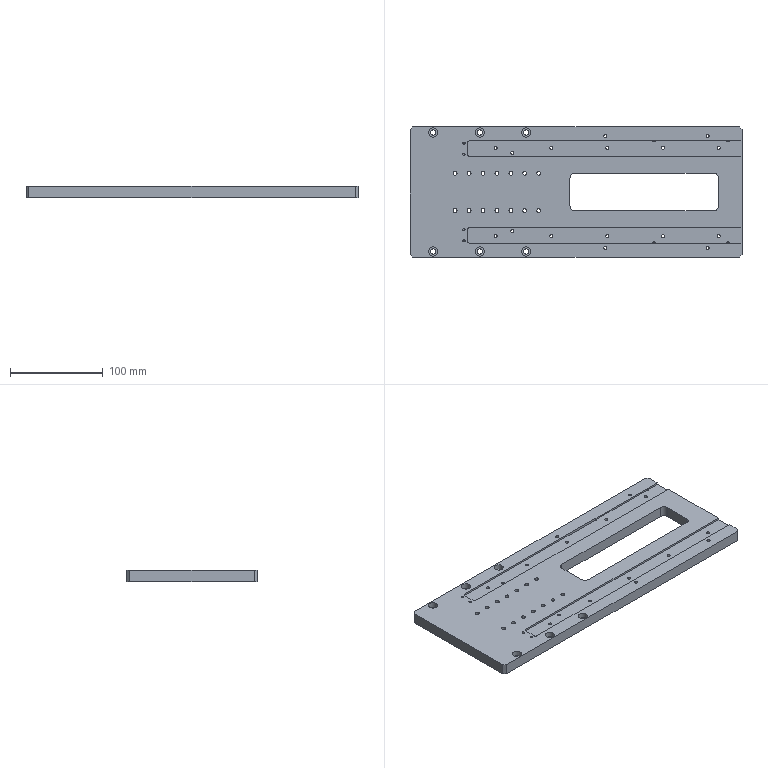NC program | NX | posted with a generic post | part box 357 x 140 x 12 mm
Lines 5825 to 6551 of 6551:
(PLANAR_MILL_COPY_COPY_COPY , TOOL : D6A45)
N11630 T01 M6
N11632 G54
N11634 G17 G0 G90 X-60.247 Y-0.314 B0. C0. S8500 M3
N11636 G43 Z30. H1
N11638 Z0.5
N11640 G94 G1 Z-1. F1250.
N11642 X-60.866 Y-1.1
N11644 G3 X-60. Y-1.6 R1.
N11646 X-58.4 Y0. R1.6
N11648 X-60. Y-1.6 R-1.6
N11650 X-59.134 Y-1.1 R1.
N11652 G1 X-59.753 Y-0.314
N11654 Z0.5
N11656 G0 Z30.
N11658 X-23.688 Y-0.13
N11660 Z0.5
N11662 G1 X-23.692 Y-0.302 Z0.454
N11664 X-23.358 Y-0.881 Z0.275
N11666 X-22.77 Y-1.2 Z0.095
N11668 X-22.23 Z-0.049
N11670 X-21.642 Y-0.881 Z-0.228
N11672 X-21.308 Y-0.302 Z-0.408
N11674 X-21.326 Y0.366 Z-0.587
N11676 X-21.596 Y0.834 Z-0.731
N11678 X-22.23 Y1.2 Z-0.928
N11680 X-22.5 Z-1.
N11682 G3 X-23.7 Y0. R1.2
N11684 X-22.5 Y1.2 R-1.2
N11686 X-23.366 Y0.7 R1.
N11688 G1 Z0.5
N11690 G0 Z30.
N11692 X23.688 Y0.13
N11694 Z0.5
N11696 G1 X23.692 Y0.302 Z0.454
N11698 X23.358 Y0.881 Z0.275
N11700 X22.77 Y1.2 Z0.095
N11702 X22.23 Z-0.049
N11704 X21.642 Y0.881 Z-0.228
N11706 X21.308 Y0.302 Z-0.408
N11708 X21.326 Y-0.366 Z-0.587
N11710 X21.596 Y-0.834 Z-0.731
N11712 X22.23 Y-1.2 Z-0.928
N11714 X22.5 Z-1.
N11716 G3 X23.7 Y0. R1.2
N11718 X22.5 Y-1.2 R-1.2
N11720 X23.366 Y-0.7 R1.
N11722 G1 Z0.5
N11724 G0 Z30.
N11726 X60.626 Y0.38
N11728 Z0.5
N11730 G1 Z-1.
N11732 X60.866 Y1.1
N11734 G3 X60. Y1.6 R1.
N11736 G1 X59.5
N11738 G3 X57.9 Y0. R1.6
N11740 X59.5 Y-1.6 R1.6
N11742 G1 X60.5
N11744 G3 X62.1 Y0. R1.6
N11746 X60.5 Y1.6 R1.6
N11748 G1 X60.
N11750 G3 X59.134 Y1.1 R1.
N11752 G1 X59.374 Y0.38
N11754 Z0.5
N11756 G0 Z30.
N11758 M5
(刀补 , TOOL : D3)
N11760 T16 M6
N11762 G54
N11764 G17 G0 G90 X-60.108 Y-0.333 B0. C0. S9500 M3
N11766 G43 Z30. H16
N11768 Z-1.
N11770 G94 G1 Z-2. F1000.
N11772 G41 X-60.26 Y-0.8 D16
N11774 G3 X-60. Y-0.95 R0.3
N11776 X-59.05 Y0. R0.95 F1200.
N11778 X-60. Y-0.95 R-0.95
N11780 G1 X-59.853 Y-0.932 Z-2.05
N11782 X-59.79 Y-0.917 Z-2.072
N11784 X-59.7 Y-0.894 Z-2.103
N11786 X-59.657 Y-0.878 Z-2.119
N11788 X-59.59 Y-0.847 Z-2.143
N11790 X-59.506 Y-0.803 Z-2.176
N11792 X-59.448 Y-0.762 Z-2.2
N11794 X-59.411 Y-0.736 Z-2.215
N11796 X-59.353 Y-0.683 Z-2.241
N11798 X-59.303 Y-0.633 Z-2.265
N11800 X-59.262 Y-0.585 Z-2.287
N11802 X-59.212 Y-0.515 Z-2.316
N11804 X-59.187 Y-0.479 Z-2.331
N11806 X-59.173 Y-0.453 Z-2.341
N11808 X-59.147 Y-0.398 Z-2.361
N11810 X-59.107 Y-0.305 Z-2.395
N11812 X-59.089 Y-0.234 Z-2.42
N11814 X-59.077 Y-0.19 Z-2.436
N11816 X-59.064 Y-0.104 Z-2.465
N11818 X-59.059 Y-0.03 Z-2.49
N11820 Y0.029 Z-2.51
N11822 X-59.066 Y0.117 Z-2.54
N11824 X-59.07 Y0.161 Z-2.555
N11826 X-59.077 Y0.19 Z-2.565
N11828 X-59.092 Y0.246 Z-2.584
N11830 X-59.128 Y0.356 Z-2.623
N11832 X-59.163 Y0.432 Z-2.652
N11834 X-59.185 Y0.477 Z-2.669
N11836 X-59.262 Y0.587 Z-2.714
N11838 X-59.287 Y0.617 Z-2.727
N11840 X-59.341 Y0.672 Z-2.753
N11842 X-59.425 Y0.746 Z-2.791
N11844 X-59.493 Y0.793 Z-2.819
N11846 X-59.539 Y0.822 Z-2.838
N11848 X-59.624 Y0.863 Z-2.869
N11850 X-59.667 Y0.882 Z-2.885
N11852 X-59.701 Y0.894 Z-2.897
N11854 X-59.771 Y0.913 Z-2.922
N11856 X-59.88 Y0.934 Z-2.959
N11858 X-59.963 Y0.941 Z-2.988
N11860 X-60.018 Y0.943 Z-3.006
N11862 X-60.159 Y0.93 Z-3.054
N11864 X-60.194 Y0.922 Z-3.066
N11866 X-60.264 Y0.903 Z-3.091
N11868 X-60.366 Y0.867 Z-3.127
N11870 X-60.441 Y0.833 Z-3.155
N11872 X-60.492 Y0.804 Z-3.175
N11874 X-60.568 Y0.751 Z-3.206
N11876 X-60.605 Y0.725 Z-3.222
N11878 X-60.678 Y0.652 Z-3.256
N11880 X-60.748 Y0.572 Z-3.292
N11882 X-60.794 Y0.507 Z-3.319
N11884 X-60.823 Y0.461 Z-3.338
N11886 X-60.861 Y0.38 Z-3.368
N11888 X-60.88 Y0.339 Z-3.383
N11890 X-60.892 Y0.306 Z-3.395
N11892 X-60.91 Y0.238 Z-3.419
N11894 X-60.933 Y0.13 Z-3.456
N11896 X-60.94 Y0.05 Z-3.483
N11898 X-60.944 Y0. Z-3.5
N11900 X-60.937 Y-0.083 Z-3.528
N11902 X-60.93 Y-0.163 Z-3.555
N11904 X-60.91 Y-0.238 Z-3.581
N11906 X-60.877 Y-0.345 Z-3.619
N11908 X-60.844 Y-0.417 Z-3.646
N11910 X-60.822 Y-0.461 Z-3.663
N11912 X-60.774 Y-0.535 Z-3.692
N11914 X-60.728 Y-0.6 Z-3.719
N11916 X-60.678 Y-0.652 Z-3.744
N11918 X-60.596 Y-0.73 Z-3.782
N11920 X-60.531 Y-0.776 Z-3.809
N11922 X-60.492 Y-0.804 Z-3.825
N11924 X-60.413 Y-0.845 Z-3.855
N11926 X-60.335 Y-0.881 Z-3.884
N11928 X-60.255 Y-0.906 Z-3.913
N11930 X-60.128 Y-0.933 Z-3.956
N11932 X-60. Y-0.95 Z-4.
N11934 X-59.854 Y-0.931 Z-4.05
N11936 X-59.79 Y-0.917 Z-4.072
N11938 X-59.701 Y-0.893 Z-4.103
N11940 X-59.657 Y-0.878 Z-4.118
N11942 X-59.591 Y-0.847 Z-4.143
N11944 X-59.505 Y-0.802 Z-4.176
N11946 X-59.448 Y-0.761 Z-4.2
N11948 X-59.411 Y-0.736 Z-4.215
N11950 X-59.354 Y-0.684 Z-4.241
N11952 X-59.304 Y-0.634 Z-4.265
N11954 X-59.262 Y-0.585 Z-4.287
N11956 X-59.187 Y-0.48 Z-4.33
N11958 X-59.173 Y-0.453 Z-4.341
N11960 X-59.147 Y-0.398 Z-4.361
N11962 X-59.108 Y-0.306 Z-4.395
N11964 X-59.089 Y-0.235 Z-4.42
N11966 X-59.078 Y-0.19 Z-4.436
N11968 X-59.065 Y-0.104 Z-4.465
N11970 X-59.058 Y-0.031 Z-4.49
N11972 X-59.059 Y0.029 Z-4.51
N11974 X-59.066 Y0.119 Z-4.541
N11976 X-59.071 Y0.165 Z-4.556
N11978 X-59.092 Y0.246 Z-4.584
N11980 X-59.128 Y0.355 Z-4.623
N11982 X-59.163 Y0.431 Z-4.651
N11984 X-59.186 Y0.477 Z-4.669
N11986 X-59.262 Y0.586 Z-4.714
N11988 X-59.286 Y0.616 Z-4.727
N11990 X-59.341 Y0.671 Z-4.753
N11992 X-59.424 Y0.745 Z-4.791
N11994 X-59.492 Y0.793 Z-4.819
N11996 X-59.539 Y0.822 Z-4.838
N11998 X-59.623 Y0.862 Z-4.869
N12000 X-59.666 Y0.882 Z-4.885
N12002 X-59.7 Y0.893 Z-4.897
N12004 X-59.771 Y0.912 Z-4.922
N12006 X-59.88 Y0.933 Z-4.959
N12008 X-59.962 Y0.941 Z-4.987
N12010 X-60.018 Y0.942 Z-5.006
N12012 X-60.162 Y0.93 Z-5.055
N12014 X-60.196 Y0.922 Z-5.067
N12016 X-60.264 Y0.903 Z-5.091
N12018 X-60.368 Y0.866 Z-5.128
N12020 X-60.443 Y0.831 Z-5.156
N12022 X-60.492 Y0.804 Z-5.175
N12024 X-60.605 Y0.725 Z-5.221
N12026 X-60.678 Y0.652 Z-5.256
N12028 X-60.747 Y0.573 Z-5.292
N12030 X-60.793 Y0.507 Z-5.319
N12032 X-60.822 Y0.461 Z-5.338
N12034 X-60.861 Y0.38 Z-5.368
N12036 X-60.88 Y0.34 Z-5.383
N12038 X-60.891 Y0.306 Z-5.395
N12040 X-60.91 Y0.238 Z-5.419
N12042 X-60.933 Y0.13 Z-5.456
N12044 X-60.94 Y0.051 Z-5.483
N12046 X-60.944 Y0. Z-5.5
N12048 X-60.937 Y-0.083 Z-5.528
N12050 X-60.93 Y-0.163 Z-5.555
N12052 X-60.91 Y-0.238 Z-5.581
N12054 X-60.878 Y-0.344 Z-5.619
N12056 X-60.844 Y-0.417 Z-5.646
N12058 X-60.822 Y-0.461 Z-5.663
N12060 X-60.774 Y-0.534 Z-5.692
N12062 X-60.729 Y-0.599 Z-5.719
N12064 X-60.678 Y-0.652 Z-5.744
N12066 X-60.597 Y-0.73 Z-5.782
N12068 X-60.532 Y-0.776 Z-5.809
N12070 X-60.492 Y-0.804 Z-5.825
N12072 X-60.412 Y-0.846 Z-5.856
N12074 X-60.333 Y-0.882 Z-5.885
N12076 X-60.255 Y-0.905 Z-5.913
N12078 X-60.128 Y-0.932 Z-5.956
N12080 X-60. Y-0.95 Z-6.
N12082 X-59.854 Y-0.931 Z-6.05
N12084 X-59.79 Y-0.917 Z-6.072
N12086 X-59.701 Y-0.893 Z-6.103
N12088 X-59.658 Y-0.878 Z-6.118
N12090 X-59.591 Y-0.847 Z-6.143
N12092 X-59.506 Y-0.802 Z-6.175
N12094 X-59.449 Y-0.762 Z-6.199
N12096 X-59.411 Y-0.736 Z-6.215
N12098 X-59.352 Y-0.682 Z-6.242
N12100 X-59.302 Y-0.633 Z-6.266
N12102 X-59.262 Y-0.585 Z-6.287
N12104 X-59.186 Y-0.477 Z-6.331
N12106 X-59.173 Y-0.451 Z-6.341
N12108 X-59.148 Y-0.398 Z-6.361
N12110 X-59.108 Y-0.307 Z-6.395
N12112 X-59.09 Y-0.236 Z-6.419
N12114 X-59.078 Y-0.19 Z-6.436
N12116 X-59.065 Y-0.105 Z-6.464
N12118 X-59.059 Y-0.032 Z-6.489
N12120 Y0.029 Z-6.51
N12122 X-59.066 Y0.119 Z-6.54
N12124 X-59.07 Y0.164 Z-6.556
N12126 X-59.092 Y0.246 Z-6.584
N12128 X-59.129 Y0.357 Z-6.624
N12130 X-59.164 Y0.432 Z-6.652
N12132 X-59.186 Y0.477 Z-6.669
N12134 X-59.262 Y0.585 Z-6.714
N12136 X-59.286 Y0.616 Z-6.727
N12138 X-59.341 Y0.671 Z-6.753
N12140 X-59.424 Y0.745 Z-6.79
N12142 X-59.492 Y0.792 Z-6.819
N12144 X-59.539 Y0.822 Z-6.838
N12146 X-59.623 Y0.862 Z-6.869
N12148 X-59.665 Y0.881 Z-6.884
N12150 X-59.7 Y0.893 Z-6.897
N12152 X-59.771 Y0.912 Z-6.922
N12154 X-59.879 Y0.934 Z-6.959
N12156 X-59.962 Y0.941 Z-6.987
N12158 X-60.018 Y0.942 Z-7.006
N12160 X-60.161 Y0.93 Z-7.055
N12162 X-60.195 Y0.921 Z-7.067
N12164 X-60.264 Y0.903 Z-7.091
N12166 X-60.367 Y0.866 Z-7.127
N12168 X-60.442 Y0.831 Z-7.156
N12170 X-60.492 Y0.804 Z-7.175
N12172 X-60.604 Y0.726 Z-7.221
N12174 X-60.629 Y0.702 Z-7.233
N12176 X-60.678 Y0.652 Z-7.256
N12178 X-60.748 Y0.571 Z-7.292
N12180 X-60.794 Y0.505 Z-7.32
N12182 X-60.822 Y0.461 Z-7.338
N12184 X-60.86 Y0.381 Z-7.367
N12186 X-60.879 Y0.34 Z-7.382
N12188 X-60.892 Y0.307 Z-7.395
N12190 X-60.91 Y0.238 Z-7.419
N12192 X-60.932 Y0.128 Z-7.457
N12194 X-60.939 Y0.048 Z-7.484
N12196 X-60.943 Y0. Z-7.5
N12198 X-60.937 Y-0.082 Z-7.528
N12200 X-60.93 Y-0.162 Z-7.555
N12202 X-60.91 Y-0.238 Z-7.581
N12204 X-60.878 Y-0.344 Z-7.619
N12206 X-60.843 Y-0.416 Z-7.646
N12208 X-60.822 Y-0.461 Z-7.663
N12210 X-60.775 Y-0.533 Z-7.692
N12212 X-60.729 Y-0.599 Z-7.719
N12214 X-60.678 Y-0.652 Z-7.744
N12216 X-60.597 Y-0.729 Z-7.781
N12218 X-60.532 Y-0.775 Z-7.808
N12220 X-60.492 Y-0.804 Z-7.825
N12222 X-60.412 Y-0.845 Z-7.856
N12224 X-60.334 Y-0.882 Z-7.885
N12226 X-60.255 Y-0.905 Z-7.913
N12228 X-60.128 Y-0.932 Z-7.956
N12230 X-60. Y-0.95 Z-8.
N12232 X-59.855 Y-0.931 Z-8.049
N12234 X-59.79 Y-0.917 Z-8.072
N12236 X-59.702 Y-0.893 Z-8.102
N12238 X-59.659 Y-0.878 Z-8.118
N12240 X-59.591 Y-0.847 Z-8.143
N12242 X-59.507 Y-0.803 Z-8.175
N12244 X-59.45 Y-0.762 Z-8.199
N12246 X-59.411 Y-0.735 Z-8.215
N12248 X-59.353 Y-0.683 Z-8.242
N12250 X-59.303 Y-0.633 Z-8.265
N12252 X-59.262 Y-0.585 Z-8.287
N12254 X-59.212 Y-0.514 Z-8.316
N12256 X-59.187 Y-0.478 Z-8.331
N12258 X-59.173 Y-0.451 Z-8.341
N12260 X-59.148 Y-0.398 Z-8.361
N12262 X-59.109 Y-0.307 Z-8.394
N12264 X-59.09 Y-0.237 Z-8.419
N12266 X-59.078 Y-0.19 Z-8.436
N12268 X-59.065 Y-0.103 Z-8.465
N12270 X-59.059 Y-0.03 Z-8.49
N12272 Y0.029 Z-8.51
N12274 X-59.066 Y0.118 Z-8.54
N12276 X-59.07 Y0.163 Z-8.555
N12278 X-59.077 Y0.19 Z-8.565
N12280 X-59.092 Y0.246 Z-8.584
N12282 X-59.129 Y0.357 Z-8.624
N12284 X-59.164 Y0.432 Z-8.652
N12286 X-59.186 Y0.477 Z-8.669
N12288 X-59.236 Y0.549 Z-8.698
N12290 X-59.285 Y0.615 Z-8.727
N12292 X-59.341 Y0.671 Z-8.753
N12294 X-59.426 Y0.746 Z-8.791
N12296 X-59.494 Y0.794 Z-8.819
N12298 X-59.539 Y0.822 Z-8.838
N12300 X-59.625 Y0.862 Z-8.869
N12302 X-59.668 Y0.882 Z-8.885
N12304 X-59.702 Y0.893 Z-8.898
N12306 X-59.771 Y0.912 Z-8.922
N12308 X-59.879 Y0.933 Z-8.959
N12310 X-59.961 Y0.94 Z-8.987
N12312 X-60.018 Y0.942 Z-9.006
N12314 X-60.112 Y0.934 Z-9.038
N12316 X-60.16 Y0.93 Z-9.054
N12318 X-60.194 Y0.921 Z-9.066
N12320 X-60.264 Y0.903 Z-9.091
N12322 X-60.367 Y0.867 Z-9.127
N12324 X-60.441 Y0.831 Z-9.155
N12326 X-60.492 Y0.804 Z-9.175
N12328 X-60.603 Y0.726 Z-9.221
N12330 X-60.628 Y0.702 Z-9.232
N12332 X-60.678 Y0.652 Z-9.256
N12334 X-60.748 Y0.572 Z-9.292
N12336 X-60.793 Y0.506 Z-9.319
N12338 X-60.822 Y0.461 Z-9.338
N12340 X-60.86 Y0.381 Z-9.367
N12342 X-60.879 Y0.341 Z-9.382
N12344 X-60.891 Y0.307 Z-9.394
N12346 X-60.91 Y0.237 Z-9.419
N12348 X-60.932 Y0.128 Z-9.456
N12350 X-60.94 Y0.049 Z-9.483
N12352 X-60.943 Y0. Z-9.5
N12354 X-60.936 Y-0.084 Z-9.529
N12356 X-60.93 Y-0.164 Z-9.556
N12358 X-60.91 Y-0.237 Z-9.581
N12360 X-60.876 Y-0.346 Z-9.62
N12362 X-60.843 Y-0.418 Z-9.647
N12364 X-60.822 Y-0.461 Z-9.663
N12366 X-60.774 Y-0.535 Z-9.693
N12368 X-60.728 Y-0.6 Z-9.72
N12370 X-60.678 Y-0.652 Z-9.744
N12372 X-60.595 Y-0.731 Z-9.782
N12374 X-60.53 Y-0.777 Z-9.809
N12376 X-60.492 Y-0.804 Z-9.825
N12378 X-60.413 Y-0.845 Z-9.855
N12380 X-60.335 Y-0.881 Z-9.885
N12382 X-60.255 Y-0.905 Z-9.913
N12384 X-60.128 Y-0.933 Z-9.956
N12386 X-60. Y-0.95 Z-10.
N12388 G3 X-59.05 Y0. R0.95
N12390 X-60. Y-0.95 R-0.95
N12392 X-59.74 Y-0.8 R0.3
N12394 G40
N12396 G1 X-59.892 Y-0.333
N12398 Z-9.
N12400 G0 Z30.
N12402 X59.446 Y-0.255
N12404 Z-1.
N12406 G1 Z-2. F1000.
N12408 G41 X59.48 Y-0.349
N12410 X59.74 Y-0.8
N12412 G3 X60. Y-0.95 R0.3
N12414 G1 X60.5 F1200.
N12416 G3 X61.45 Y0. R0.95
N12418 X60.5 Y0.95 R0.95
N12420 G1 X59.5
N12422 G3 X58.55 Y0. R0.95
N12424 X59.5 Y-0.95 R0.95
N12426 G1 X60.
N12428 X60.25 Z-2.063
N12430 X60.5 Y-0.944 Z-2.126
N12432 X60.609 Y-0.935 Z-2.153
N12434 X60.664 Y-0.93 Z-2.167
N12436 X60.743 Y-0.909 Z-2.188
N12438 X60.852 Y-0.874 Z-2.217
N12440 X60.926 Y-0.839 Z-2.238
N12442 X60.971 Y-0.818 Z-2.25
N12444 X61.041 Y-0.77 Z-2.272
N12446 X61.108 Y-0.722 Z-2.293
N12448 X61.164 Y-0.666 Z-2.312
N12450 X61.242 Y-0.581 Z-2.341
N12452 X61.289 Y-0.514 Z-2.362
N12454 X61.316 Y-0.474 Z-2.375
N12456 X61.353 Y-0.397 Z-2.396
N12458 X61.388 Y-0.322 Z-2.417
N12460 X61.408 Y-0.246 Z-2.437
N12462 X61.433 Y-0.131 Z-2.467
N12464 X61.44 Y-0.049 Z-2.487
N12466 X61.444 Y-0.002 Z-2.499
N12468 X61.437 Y0.083 Z-2.521
N12470 X61.43 Y0.165 Z-2.542
N12472 X61.409 Y0.242 Z-2.562
N12474 X61.373 Y0.353 Z-2.591
N12476 X61.339 Y0.428 Z-2.612
N12478 X61.318 Y0.471 Z-2.624
N12480 X61.27 Y0.541 Z-2.646
N12482 X61.222 Y0.609 Z-2.667
N12484 X61.166 Y0.665 Z-2.687
N12486 X61.079 Y0.743 Z-2.716
N12488 X61.012 Y0.79 Z-2.737
N12490 X60.973 Y0.817 Z-2.749
N12492 X60.895 Y0.854 Z-2.771
N12494 X60.82 Y0.888 Z-2.792
N12496 X60.744 Y0.909 Z-2.812
N12498 X60.623 Y0.934 Z-2.843
N12500 X60.5 Y0.944 Z-2.874
N12502 X60. Y0.95 Z-3.
N12504 X59.5 Y0.944 Z-3.126
N12506 X59.39 Y0.935 Z-3.154
N12508 X59.334 Y0.93 Z-3.168
N12510 X59.249 Y0.907 Z-3.19
N12512 X59.139 Y0.87 Z-3.219
N12514 X59.063 Y0.834 Z-3.241
N12516 X59.014 Y0.808 Z-3.255
N12518 X58.932 Y0.751 Z-3.28
N12520 X58.891 Y0.721 Z-3.293
N12522 X58.865 Y0.696 Z-3.302
N12524 X58.814 Y0.644 Z-3.32
N12526 X58.743 Y0.559 Z-3.348
N12528 X58.694 Y0.488 Z-3.37
N12530 X58.664 Y0.433 Z-3.386
N12532 X58.617 Y0.332 Z-3.414
N12534 X58.593 Y0.25 Z-3.436
N12536 X58.577 Y0.189 Z-3.452
N12538 X58.564 Y0.09 Z-3.477
N12540 X58.556 Y0.004 Z-3.499
N12542 X58.562 Y-0.069 Z-3.517
N12544 X58.578 Y-0.192 Z-3.549
N12546 X58.6 Y-0.275 Z-3.571
N12548 X58.613 Y-0.323 Z-3.583
N12550 X58.67 Y-0.447 Z-3.618
N12552 X58.69 Y-0.483 Z-3.628
N12554 X58.737 Y-0.551 Z-3.649
N12556 X58.806 Y-0.636 Z-3.676
N12558 X58.867 Y-0.697 Z-3.698
N12560 X58.915 Y-0.738 Z-3.715
N12562 X58.981 Y-0.785 Z-3.735
N12564 X59.04 Y-0.824 Z-3.753
N12566 X59.094 Y-0.849 Z-3.768
N12568 X59.19 Y-0.891 Z-3.794
N12570 X59.292 Y-0.917 Z-3.821
N12572 X59.395 Y-0.935 Z-3.848
N12574 X59.5 Y-0.944 Z-3.874
N12576 X59.75 Y-0.95 Z-3.937
N12578 X60. Z-4.
N12580 X60.25 Z-4.063
N12582 X60.5 Y-0.944 Z-4.126
N12584 X60.61 Y-0.935 Z-4.153
N12586 X60.664 Y-0.93 Z-4.167
N12588 X60.743 Y-0.909 Z-4.188
N12590 X60.854 Y-0.873 Z-4.217
N12592 X60.928 Y-0.838 Z-4.238
N12594 X60.971 Y-0.818 Z-4.25
N12596 X61.041 Y-0.77 Z-4.272
N12598 X61.108 Y-0.723 Z-4.292
N12600 X61.164 Y-0.666 Z-4.312
N12602 X61.242 Y-0.58 Z-4.342
N12604 X61.289 Y-0.513 Z-4.363
N12606 X61.316 Y-0.474 Z-4.375
N12608 X61.353 Y-0.397 Z-4.396
N12610 X61.387 Y-0.323 Z-4.417
N12612 X61.408 Y-0.246 Z-4.437
N12614 X61.433 Y-0.132 Z-4.466
N12616 X61.44 Y-0.05 Z-4.487
N12618 X61.444 Y-0.002 Z-4.499
N12620 X61.437 Y0.082 Z-4.521
N12622 X61.43 Y0.164 Z-4.542
N12624 X61.409 Y0.242 Z-4.562
N12626 X61.373 Y0.353 Z-4.591
N12628 X61.339 Y0.427 Z-4.612
N12630 X61.318 Y0.471 Z-4.624
N12632 X61.27 Y0.541 Z-4.646
N12634 X61.223 Y0.608 Z-4.667
N12636 X61.166 Y0.664 Z-4.687
N12638 X61.079 Y0.743 Z-4.716
N12640 X61.012 Y0.789 Z-4.737
N12642 X60.972 Y0.817 Z-4.749
N12644 X60.896 Y0.853 Z-4.771
N12646 X60.821 Y0.888 Z-4.792
N12648 X60.744 Y0.909 Z-4.812
N12650 X60.623 Y0.933 Z-4.843
N12652 X60.5 Y0.944 Z-4.874
N12654 X60. Y0.95 Z-5.
N12656 X59.5 Y0.944 Z-5.126
N12658 X59.389 Y0.935 Z-5.154
N12660 X59.334 Y0.929 Z-5.168
N12662 X59.249 Y0.906 Z-5.19
N12664 X59.14 Y0.87 Z-5.219
N12666 X59.063 Y0.834 Z-5.241
N12668 X59.014 Y0.808 Z-5.255
N12670 X58.933 Y0.751 Z-5.28
N12672 X58.892 Y0.722 Z-5.292
N12674 X58.866 Y0.696 Z-5.302
N12676 X58.814 Y0.644 Z-5.32
N12678 X58.744 Y0.559 Z-5.348
N12680 X58.694 Y0.489 Z-5.37
N12682 X58.664 Y0.433 Z-5.386
N12684 X58.617 Y0.331 Z-5.414
N12686 X58.593 Y0.248 Z-5.436
N12688 X58.578 Y0.189 Z-5.452
N12690 X58.564 Y0.091 Z-5.477
N12692 X58.556 Y0.004 Z-5.499
N12694 X58.562 Y-0.069 Z-5.517
N12696 X58.577 Y-0.192 Z-5.548
N12698 X58.6 Y-0.275 Z-5.57
N12700 X58.613 Y-0.323 Z-5.583
N12702 X58.653 Y-0.408 Z-5.607
N12704 X58.673 Y-0.45 Z-5.619
N12706 X58.692 Y-0.485 Z-5.629
N12708 X58.737 Y-0.55 Z-5.649
N12710 X58.805 Y-0.636 Z-5.676
N12712 X58.866 Y-0.697 Z-5.698
N12714 X58.915 Y-0.738 Z-5.715
N12716 X58.983 Y-0.787 Z-5.736
N12718 X59.018 Y-0.81 Z-5.746
N12720 X59.042 Y-0.824 Z-5.753
N12722 X59.094 Y-0.848 Z-5.768
N12724 X59.19 Y-0.891 Z-5.794
N12726 X59.292 Y-0.917 Z-5.821
N12728 X59.395 Y-0.935 Z-5.848
N12730 X59.5 Y-0.944 Z-5.874
N12732 X59.75 Y-0.95 Z-5.937
N12734 X60. Z-6.
N12736 X60.25 Z-6.063
N12738 X60.5 Y-0.944 Z-6.126
N12740 X60.61 Y-0.935 Z-6.153
N12742 X60.665 Y-0.93 Z-6.167
N12744 X60.743 Y-0.909 Z-6.188
N12746 X60.854 Y-0.872 Z-6.217
N12748 X60.928 Y-0.838 Z-6.238
N12750 X60.971 Y-0.818 Z-6.25
N12752 X61.04 Y-0.77 Z-6.272
N12754 X61.107 Y-0.723 Z-6.292
N12756 X61.164 Y-0.666 Z-6.312
N12758 X61.242 Y-0.58 Z-6.342
N12760 X61.288 Y-0.513 Z-6.362
N12762 X61.316 Y-0.474 Z-6.375
N12764 X61.352 Y-0.398 Z-6.396
N12766 X61.387 Y-0.323 Z-6.417
N12768 X61.408 Y-0.246 Z-6.437
N12770 X61.432 Y-0.132 Z-6.466
N12772 X61.439 Y-0.051 Z-6.487
N12774 X61.443 Y-0.002 Z-6.499
N12776 X61.437 Y0.082 Z-6.521
N12778 X61.43 Y0.164 Z-6.542
N12780 X61.409 Y0.242 Z-6.562
N12782 X61.373 Y0.352 Z-6.591
N12784 X61.339 Y0.426 Z-6.612
N12786 X61.318 Y0.47 Z-6.624
N12788 X61.27 Y0.54 Z-6.646
N12790 X61.223 Y0.607 Z-6.667
N12792 X61.166 Y0.664 Z-6.687
N12794 X61.08 Y0.742 Z-6.716
N12796 X61.012 Y0.789 Z-6.737
N12798 X60.972 Y0.817 Z-6.749
N12800 X60.896 Y0.853 Z-6.771
N12802 X60.822 Y0.887 Z-6.791
N12804 X60.744 Y0.908 Z-6.812
N12806 X60.623 Y0.933 Z-6.843
N12808 X60.5 Y0.943 Z-6.874
N12810 X60. Y0.95 Z-7.
N12812 X59.5 Y0.943 Z-7.126
N12814 X59.389 Y0.934 Z-7.154
N12816 X59.334 Y0.929 Z-7.168
N12818 X59.249 Y0.906 Z-7.19
N12820 X59.14 Y0.87 Z-7.219
N12822 X59.064 Y0.834 Z-7.24
N12824 X59.015 Y0.808 Z-7.255
N12826 X58.893 Y0.723 Z-7.292
N12828 X58.814 Y0.644 Z-7.32
N12830 X58.744 Y0.56 Z-7.348
N12832 X58.694 Y0.489 Z-7.37
N12834 X58.664 Y0.433 Z-7.386
N12836 X58.617 Y0.332 Z-7.414
N12838 X58.593 Y0.249 Z-7.436
N12840 X58.578 Y0.189 Z-7.452
N12842 X58.564 Y0.089 Z-7.477
N12844 X58.556 Y0.003 Z-7.499
N12846 X58.562 Y-0.069 Z-7.517
N12848 X58.577 Y-0.191 Z-7.548
N12850 X58.6 Y-0.274 Z-7.57
N12852 X58.614 Y-0.323 Z-7.583
N12854 X58.652 Y-0.407 Z-7.607
N12856 X58.691 Y-0.485 Z-7.629
N12858 X58.737 Y-0.55 Z-7.649
N12860 X58.807 Y-0.636 Z-7.677
N12862 X58.868 Y-0.697 Z-7.699
N12864 X58.915 Y-0.738 Z-7.715
N12866 X58.983 Y-0.786 Z-7.736
N12868 X59.017 Y-0.81 Z-7.746
N12870 X59.042 Y-0.824 Z-7.753
N12872 X59.094 Y-0.848 Z-7.768
N12874 X59.179 Y-0.887 Z-7.791
N12876 X59.246 Y-0.905 Z-7.809
N12878 X59.292 Y-0.917 Z-7.821
N12880 X59.395 Y-0.934 Z-7.848
N12882 X59.5 Y-0.943 Z-7.874
N12884 X59.75 Y-0.95 Z-7.937
N12886 X60. Z-8.
N12888 X60.25 Z-8.063
N12890 X60.5 Y-0.943 Z-8.126
N12892 X60.61 Y-0.934 Z-8.154
N12894 X60.665 Y-0.929 Z-8.167
N12896 X60.743 Y-0.909 Z-8.188
N12898 X60.853 Y-0.872 Z-8.217
N12900 X60.927 Y-0.838 Z-8.238
N12902 X60.971 Y-0.817 Z-8.25
N12904 X61.039 Y-0.77 Z-8.271
N12906 X61.106 Y-0.723 Z-8.292
N12908 X61.164 Y-0.666 Z-8.312
N12910 X61.241 Y-0.581 Z-8.341
N12912 X61.288 Y-0.514 Z-8.362
N12914 X61.316 Y-0.473 Z-8.375
N12916 X61.352 Y-0.398 Z-8.396
N12918 X61.386 Y-0.324 Z-8.417
N12920 X61.408 Y-0.246 Z-8.437
N12922 X61.433 Y-0.133 Z-8.466
N12924 X61.439 Y-0.051 Z-8.487
N12926 X61.443 Y-0.002 Z-8.499
N12928 X61.437 Y0.081 Z-8.521
N12930 X61.429 Y0.163 Z-8.541
N12932 X61.409 Y0.242 Z-8.562
N12934 X61.373 Y0.351 Z-8.591
N12936 X61.339 Y0.426 Z-8.612
N12938 X61.318 Y0.47 Z-8.624
N12940 X61.268 Y0.542 Z-8.646
N12942 X61.221 Y0.609 Z-8.667
N12944 X61.166 Y0.664 Z-8.687
N12946 X61.08 Y0.741 Z-8.716
N12948 X61.013 Y0.789 Z-8.737
N12950 X60.972 Y0.817 Z-8.749
N12952 X60.894 Y0.853 Z-8.771
N12954 X60.819 Y0.888 Z-8.792
N12956 X60.744 Y0.908 Z-8.812
N12958 X60.623 Y0.933 Z-8.843
N12960 X60.5 Y0.943 Z-8.874
N12962 X60. Y0.95 Z-9.
N12964 X59.5 Y0.943 Z-9.126
N12966 X59.389 Y0.934 Z-9.154
N12968 X59.334 Y0.929 Z-9.168
N12970 X59.249 Y0.906 Z-9.19
N12972 X59.139 Y0.869 Z-9.219
N12974 X59.063 Y0.833 Z-9.241
N12976 X59.015 Y0.808 Z-9.255
N12978 X58.894 Y0.723 Z-9.292
N12980 X58.867 Y0.697 Z-9.301
N12982 X58.814 Y0.644 Z-9.32
N12984 X58.743 Y0.559 Z-9.348
N12986 X58.694 Y0.488 Z-9.37
N12988 X58.664 Y0.433 Z-9.386
N12990 X58.618 Y0.332 Z-9.414
N12992 X58.593 Y0.25 Z-9.436
N12994 X58.578 Y0.189 Z-9.452
N12996 X58.564 Y0.09 Z-9.477
N12998 X58.557 Y0.004 Z-9.499
N13000 X58.562 Y-0.069 Z-9.517
N13002 X58.578 Y-0.19 Z-9.548
N13004 X58.6 Y-0.273 Z-9.57
N13006 X58.614 Y-0.323 Z-9.583
N13008 X58.671 Y-0.449 Z-9.618
N13010 X58.691 Y-0.484 Z-9.628
N13012 X58.738 Y-0.55 Z-9.649
N13014 X58.806 Y-0.636 Z-9.677
N13016 X58.867 Y-0.697 Z-9.698
N13018 X58.916 Y-0.738 Z-9.715
N13020 X58.983 Y-0.786 Z-9.735
N13022 X59.016 Y-0.809 Z-9.746
N13024 X59.042 Y-0.823 Z-9.753
N13026 X59.094 Y-0.848 Z-9.768
N13028 X59.178 Y-0.887 Z-9.791
N13030 X59.245 Y-0.905 Z-9.809
N13032 X59.292 Y-0.917 Z-9.821
N13034 X59.395 Y-0.935 Z-9.848
N13036 X59.5 Y-0.943 Z-9.874
N13038 X59.75 Y-0.95 Z-9.937
N13040 X60. Z-10.
N13042 X60.5
N13044 G3 X61.45 Y0. R0.95
N13046 X60.5 Y0.95 R0.95
N13048 G1 X59.5
N13050 G3 X58.55 Y0. R0.95
N13052 X59.5 Y-0.95 R0.95
N13054 G1 X60.
N13056 G3 X60.26 Y-0.8 R0.3
N13058 G1 X60.52 Y-0.349
N13060 G40
N13062 X60.554 Y-0.255
N13064 Z-9.
N13066 G0 Z30.
N13068 M5
N13070 M2